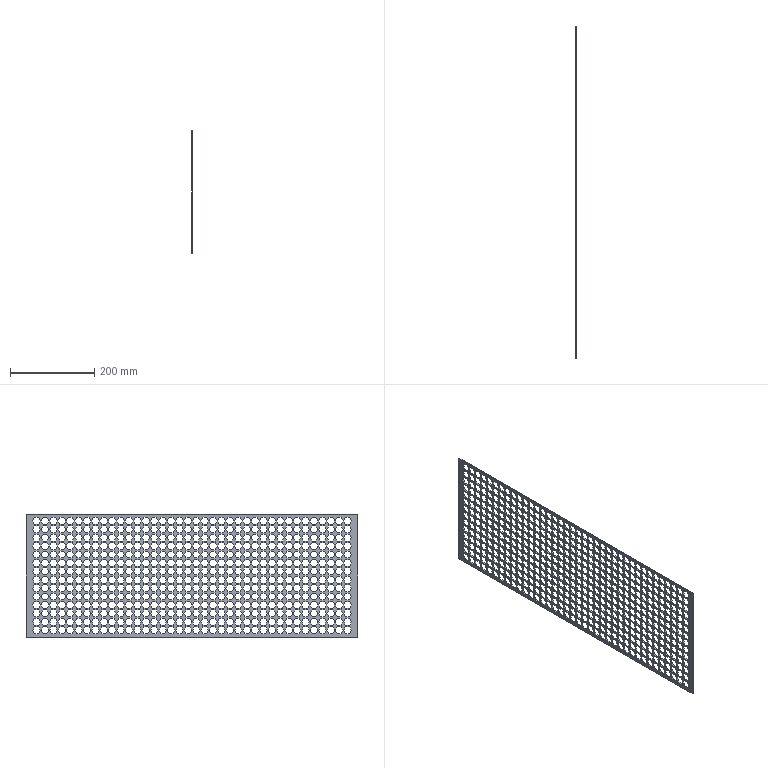Part | SolidWorks | features ICE 2, Cut 1, Extrusion 1, LPattern 1 | 1 solid | 3198 faces | volume 218859 mm3 | plane 3198